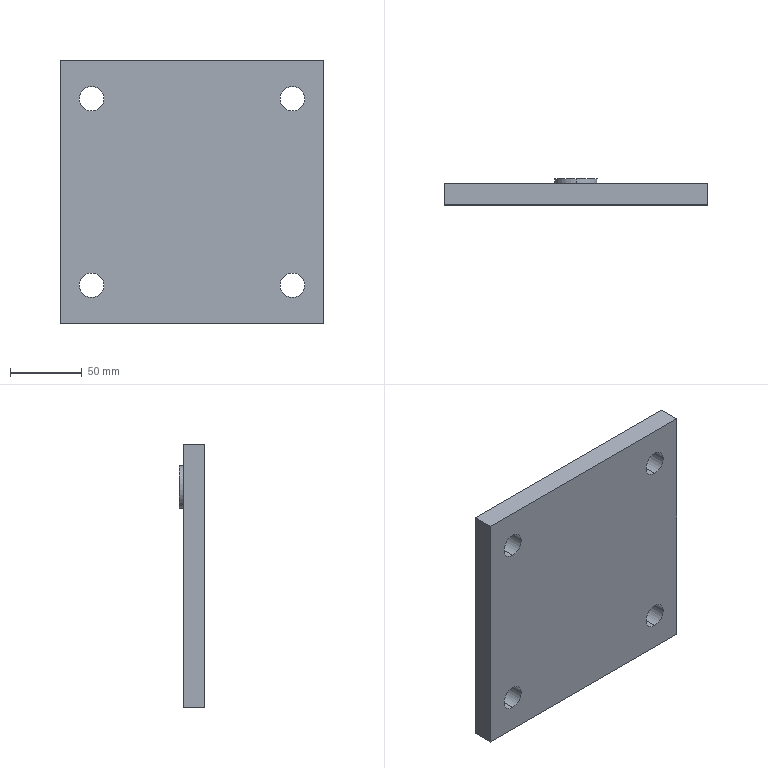Part | SolidWorks | features BaseBody 1 | 1 solid | 17 faces | box 184 x 18 x 184 mm | volume 496342 mm3 | cylinder 10 | plane 7 | commonest cylinder face diameters 17 x8 30 x2
STEP:
#1=CARTESIAN_POINT('',(70.,79.2,-206.379));
#2=VERTEX_POINT('',#1);
#3=CARTESIAN_POINT('',(70.,79.2,-223.379));
#4=VERTEX_POINT('',#3);
#5=CARTESIAN_POINT('',(70.,79.2,-214.879));
#6=DIRECTION('',(0.,-1.,0.));
#7=DIRECTION('',(0.,0.,-1.));
#8=AXIS2_PLACEMENT_3D('',#5,#6,#7);
#9=CIRCLE('',#8,8.5);
#10=EDGE_CURVE('',#2,#4,#9,.T.);
#11=ORIENTED_EDGE('',*,*,#10,.F.);
#12=CARTESIAN_POINT('',(70.,64.2,-206.379));
#13=VERTEX_POINT('',#12);
#14=CARTESIAN_POINT('',(70.,82.2,-206.379));
#15=DIRECTION('',(0.,-1.,0.));
#16=VECTOR('',#15,1000.);
#17=LINE('',#14,#16);
#18=EDGE_CURVE('',#2,#13,#17,.T.);
#19=ORIENTED_EDGE('',*,*,#18,.T.);
#20=CARTESIAN_POINT('',(70.,64.2,-223.379));
#21=VERTEX_POINT('',#20);
#22=CARTESIAN_POINT('',(70.,64.2,-214.879));
#23=DIRECTION('',(0.,-1.,0.));
#24=DIRECTION('',(0.,0.,-1.));
#25=AXIS2_PLACEMENT_3D('',#22,#23,#24);
#26=CIRCLE('',#25,8.5);
#27=EDGE_CURVE('',#13,#21,#26,.T.);
#28=ORIENTED_EDGE('',*,*,#27,.T.);
#29=CARTESIAN_POINT('',(70.,82.2,-223.379));
#30=DIRECTION('',(0.,-1.,0.));
#31=VECTOR('',#30,1000.);
#32=LINE('',#29,#31);
#33=EDGE_CURVE('',#4,#21,#32,.T.);
#34=ORIENTED_EDGE('',*,*,#33,.F.);
#35=EDGE_LOOP('',(#11,#19,#28,#34));
#36=FACE_OUTER_BOUND('',#35,.T.);
#37=CARTESIAN_POINT('',(70.,82.2,-214.879));
#38=DIRECTION('',(0.,-1.,0.));
#39=DIRECTION('',(0.,0.,-1.));
#40=AXIS2_PLACEMENT_3D('',#37,#38,#39);
#41=CYLINDRICAL_SURFACE('',#40,8.5);
#42=ADVANCED_FACE('',(#36),#41,.F.);
#43=CARTESIAN_POINT('',(70.,79.2,-76.379));
#44=VERTEX_POINT('',#43);
#45=CARTESIAN_POINT('',(70.,79.2,-93.379));
#46=VERTEX_POINT('',#45);
#47=CARTESIAN_POINT('',(70.,79.2,-84.879));
#48=DIRECTION('',(0.,-1.,0.));
#49=DIRECTION('',(0.,0.,-1.));
#50=AXIS2_PLACEMENT_3D('',#47,#48,#49);
#51=CIRCLE('',#50,8.5);
#52=EDGE_CURVE('',#44,#46,#51,.T.);
#53=ORIENTED_EDGE('',*,*,#52,.F.);
#54=CARTESIAN_POINT('',(70.,64.2,-76.379));
#55=VERTEX_POINT('',#54);
#56=CARTESIAN_POINT('',(70.,82.2,-76.379));
#57=DIRECTION('',(0.,-1.,0.));
#58=VECTOR('',#57,1000.);
#59=LINE('',#56,#58);
#60=EDGE_CURVE('',#44,#55,#59,.T.);
#61=ORIENTED_EDGE('',*,*,#60,.T.);
#62=CARTESIAN_POINT('',(70.,64.2,-93.379));
#63=VERTEX_POINT('',#62);
#64=CARTESIAN_POINT('',(70.,64.2,-84.879));
#65=DIRECTION('',(0.,-1.,0.));
#66=DIRECTION('',(0.,0.,-1.));
#67=AXIS2_PLACEMENT_3D('',#64,#65,#66);
#68=CIRCLE('',#67,8.5);
#69=EDGE_CURVE('',#55,#63,#68,.T.);
#70=ORIENTED_EDGE('',*,*,#69,.T.);
#71=CARTESIAN_POINT('',(70.,82.2,-93.379));
#72=DIRECTION('',(0.,-1.,0.));
#73=VECTOR('',#72,1000.);
#74=LINE('',#71,#73);
#75=EDGE_CURVE('',#46,#63,#74,.T.);
#76=ORIENTED_EDGE('',*,*,#75,.F.);
#77=EDGE_LOOP('',(#53,#61,#70,#76));
#78=FACE_OUTER_BOUND('',#77,.T.);
#79=CARTESIAN_POINT('',(70.,82.2,-84.879));
#80=DIRECTION('',(0.,-1.,0.));
#81=DIRECTION('',(0.,0.,-1.));
#82=AXIS2_PLACEMENT_3D('',#79,#80,#81);
#83=CYLINDRICAL_SURFACE('',#82,8.5);
#84=ADVANCED_FACE('',(#78),#83,.F.);
#85=CARTESIAN_POINT('',(-70.,79.2,-206.379));
#86=VERTEX_POINT('',#85);
#87=CARTESIAN_POINT('',(-70.,79.2,-223.379));
#88=VERTEX_POINT('',#87);
#89=CARTESIAN_POINT('',(-70.,79.2,-214.879));
#90=DIRECTION('',(0.,-1.,0.));
#91=DIRECTION('',(0.,0.,-1.));
#92=AXIS2_PLACEMENT_3D('',#89,#90,#91);
#93=CIRCLE('',#92,8.5);
#94=EDGE_CURVE('',#86,#88,#93,.T.);
#95=ORIENTED_EDGE('',*,*,#94,.F.);
#96=CARTESIAN_POINT('',(-70.,64.2,-206.379));
#97=VERTEX_POINT('',#96);
#98=CARTESIAN_POINT('',(-70.,82.2,-206.379));
#99=DIRECTION('',(0.,-1.,0.));
#100=VECTOR('',#99,1000.);
#101=LINE('',#98,#100);
#102=EDGE_CURVE('',#86,#97,#101,.T.);
#103=ORIENTED_EDGE('',*,*,#102,.T.);
#104=CARTESIAN_POINT('',(-70.,64.2,-223.379));
#105=VERTEX_POINT('',#104);
#106=CARTESIAN_POINT('',(-70.,64.2,-214.879));
#107=DIRECTION('',(0.,-1.,0.));
#108=DIRECTION('',(0.,0.,-1.));
#109=AXIS2_PLACEMENT_3D('',#106,#107,#108);
#110=CIRCLE('',#109,8.5);
#111=EDGE_CURVE('',#97,#105,#110,.T.);
#112=ORIENTED_EDGE('',*,*,#111,.T.);
#113=CARTESIAN_POINT('',(-70.,82.2,-223.379));
#114=DIRECTION('',(0.,-1.,0.));
#115=VECTOR('',#114,1000.);
#116=LINE('',#113,#115);
#117=EDGE_CURVE('',#88,#105,#116,.T.);
#118=ORIENTED_EDGE('',*,*,#117,.F.);
#119=EDGE_LOOP('',(#95,#103,#112,#118));
#120=FACE_OUTER_BOUND('',#119,.T.);
#121=CARTESIAN_POINT('',(-70.,82.2,-214.879));
#122=DIRECTION('',(0.,-1.,0.));
#123=DIRECTION('',(0.,0.,-1.));
#124=AXIS2_PLACEMENT_3D('',#121,#122,#123);
#125=CYLINDRICAL_SURFACE('',#124,8.5);
#126=ADVANCED_FACE('',(#120),#125,.F.);
#127=CARTESIAN_POINT('',(-70.,79.2,-76.379));
#128=VERTEX_POINT('',#127);
#129=CARTESIAN_POINT('',(-70.,79.2,-93.379));
#130=VERTEX_POINT('',#129);
#131=CARTESIAN_POINT('',(-70.,79.2,-84.879));
#132=DIRECTION('',(0.,-1.,0.));
#133=DIRECTION('',(0.,0.,-1.));
#134=AXIS2_PLACEMENT_3D('',#131,#132,#133);
#135=CIRCLE('',#134,8.5);
#136=EDGE_CURVE('',#128,#130,#135,.T.);
#137=ORIENTED_EDGE('',*,*,#136,.F.);
#138=CARTESIAN_POINT('',(-70.,64.2,-76.379));
#139=VERTEX_POINT('',#138);
#140=CARTESIAN_POINT('',(-70.,82.2,-76.379));
#141=DIRECTION('',(0.,-1.,0.));
#142=VECTOR('',#141,1000.);
#143=LINE('',#140,#142);
#144=EDGE_CURVE('',#128,#139,#143,.T.);
#145=ORIENTED_EDGE('',*,*,#144,.T.);
#146=CARTESIAN_POINT('',(-70.,64.2,-93.379));
#147=VERTEX_POINT('',#146);
#148=CARTESIAN_POINT('',(-70.,64.2,-84.879));
#149=DIRECTION('',(0.,-1.,0.));
#150=DIRECTION('',(0.,0.,-1.));
#151=AXIS2_PLACEMENT_3D('',#148,#149,#150);
#152=CIRCLE('',#151,8.5);
#153=EDGE_CURVE('',#139,#147,#152,.T.);
#154=ORIENTED_EDGE('',*,*,#153,.T.);
#155=CARTESIAN_POINT('',(-70.,82.2,-93.379));
#156=DIRECTION('',(0.,-1.,0.));
#157=VECTOR('',#156,1000.);
#158=LINE('',#155,#157);
#159=EDGE_CURVE('',#130,#147,#158,.T.);
#160=ORIENTED_EDGE('',*,*,#159,.F.);
#161=EDGE_LOOP('',(#137,#145,#154,#160));
#162=FACE_OUTER_BOUND('',#161,.T.);
#163=CARTESIAN_POINT('',(-70.,82.2,-84.879));
#164=DIRECTION('',(0.,-1.,0.));
#165=DIRECTION('',(0.,0.,-1.));
#166=AXIS2_PLACEMENT_3D('',#163,#164,#165);
#167=CYLINDRICAL_SURFACE('',#166,8.5);
#168=ADVANCED_FACE('',(#162),#167,.F.);
#169=CARTESIAN_POINT('',(0.,82.2,-102.879));
#170=VERTEX_POINT('',#169);
#171=CARTESIAN_POINT('',(0.,82.2,-72.879));
#172=VERTEX_POINT('',#171);
#173=CARTESIAN_POINT('',(0.,82.2,-87.879));
#174=DIRECTION('',(0.,-1.,0.));
#175=DIRECTION('',(0.,0.,-1.));
#176=AXIS2_PLACEMENT_3D('',#173,#174,#175);
#177=CIRCLE('',#176,15.);
#178=EDGE_CURVE('',#170,#172,#177,.T.);
#179=ORIENTED_EDGE('',*,*,#178,.T.);
#180=CARTESIAN_POINT('',(0.,79.2,-72.879));
#181=VERTEX_POINT('',#180);
#182=CARTESIAN_POINT('',(0.,82.2,-72.879));
#183=DIRECTION('',(0.,-1.,0.));
#184=VECTOR('',#183,1000.);
#185=LINE('',#182,#184);
#186=EDGE_CURVE('',#172,#181,#185,.T.);
#187=ORIENTED_EDGE('',*,*,#186,.T.);
#188=CARTESIAN_POINT('',(0.,79.2,-102.879));
#189=VERTEX_POINT('',#188);
#190=CARTESIAN_POINT('',(0.,79.2,-87.879));
#191=DIRECTION('',(0.,-1.,0.));
#192=DIRECTION('',(0.,0.,-1.));
#193=AXIS2_PLACEMENT_3D('',#190,#191,#192);
#194=CIRCLE('',#193,15.);
#195=EDGE_CURVE('',#189,#181,#194,.T.);
#196=ORIENTED_EDGE('',*,*,#195,.F.);
#197=CARTESIAN_POINT('',(0.,82.2,-102.879));
#198=DIRECTION('',(0.,-1.,0.));
#199=VECTOR('',#198,1000.);
#200=LINE('',#197,#199);
#201=EDGE_CURVE('',#170,#189,#200,.T.);
#202=ORIENTED_EDGE('',*,*,#201,.F.);
#203=EDGE_LOOP('',(#179,#187,#196,#202));
#204=FACE_OUTER_BOUND('',#203,.T.);
#205=CARTESIAN_POINT('',(0.,82.2,-87.879));
#206=DIRECTION('',(0.,-1.,0.));
#207=DIRECTION('',(0.,0.,-1.));
#208=AXIS2_PLACEMENT_3D('',#205,#206,#207);
#209=CYLINDRICAL_SURFACE('',#208,15.);
#210=ADVANCED_FACE('',(#204),#209,.T.);
#211=CARTESIAN_POINT('',(92.,64.2,-241.879));
#212=VERTEX_POINT('',#211);
#213=CARTESIAN_POINT('',(-92.,64.2,-241.879));
#214=VERTEX_POINT('',#213);
#215=CARTESIAN_POINT('',(0.,64.2,-241.879));
#216=DIRECTION('',(-1.,0.,0.));
#217=VECTOR('',#216,1000.);
#218=LINE('',#215,#217);
#219=EDGE_CURVE('',#212,#214,#218,.T.);
#220=ORIENTED_EDGE('',*,*,#219,.F.);
#221=CARTESIAN_POINT('',(92.,64.2,-57.879));
#222=VERTEX_POINT('',#221);
#223=CARTESIAN_POINT('',(92.,64.2,-149.879));
#224=DIRECTION('',(0.,0.,-1.));
#225=VECTOR('',#224,1000.);
#226=LINE('',#223,#225);
#227=EDGE_CURVE('',#222,#212,#226,.T.);
#228=ORIENTED_EDGE('',*,*,#227,.F.);
#229=CARTESIAN_POINT('',(-92.,64.2,-57.879));
#230=VERTEX_POINT('',#229);
#231=CARTESIAN_POINT('',(0.,64.2,-57.879));
#232=DIRECTION('',(1.,0.,0.));
#233=VECTOR('',#232,1000.);
#234=LINE('',#231,#233);
#235=EDGE_CURVE('',#230,#222,#234,.T.);
#236=ORIENTED_EDGE('',*,*,#235,.F.);
#237=CARTESIAN_POINT('',(-92.,64.2,-149.879));
#238=DIRECTION('',(0.,0.,1.));
#239=VECTOR('',#238,1000.);
#240=LINE('',#237,#239);
#241=EDGE_CURVE('',#214,#230,#240,.T.);
#242=ORIENTED_EDGE('',*,*,#241,.F.);
#243=EDGE_LOOP('',(#220,#228,#236,#242));
#244=FACE_OUTER_BOUND('',#243,.T.);
#245=CARTESIAN_POINT('',(70.,64.2,-214.879));
#246=DIRECTION('',(0.,-1.,0.));
#247=DIRECTION('',(0.,0.,-1.));
#248=AXIS2_PLACEMENT_3D('',#245,#246,#247);
#249=CIRCLE('',#248,8.5);
#250=EDGE_CURVE('',#21,#13,#249,.T.);
#251=ORIENTED_EDGE('',*,*,#250,.F.);
#252=ORIENTED_EDGE('',*,*,#27,.F.);
#253=EDGE_LOOP('',(#251,#252));
#254=FACE_BOUND('',#253,.T.);
#255=CARTESIAN_POINT('',(70.,64.2,-84.879));
#256=DIRECTION('',(0.,-1.,0.));
#257=DIRECTION('',(0.,0.,-1.));
#258=AXIS2_PLACEMENT_3D('',#255,#256,#257);
#259=CIRCLE('',#258,8.5);
#260=EDGE_CURVE('',#63,#55,#259,.T.);
#261=ORIENTED_EDGE('',*,*,#260,.F.);
#262=ORIENTED_EDGE('',*,*,#69,.F.);
#263=EDGE_LOOP('',(#261,#262));
#264=FACE_BOUND('',#263,.T.);
#265=CARTESIAN_POINT('',(-70.,64.2,-214.879));
#266=DIRECTION('',(0.,-1.,0.));
#267=DIRECTION('',(0.,0.,-1.));
#268=AXIS2_PLACEMENT_3D('',#265,#266,#267);
#269=CIRCLE('',#268,8.5);
#270=EDGE_CURVE('',#105,#97,#269,.T.);
#271=ORIENTED_EDGE('',*,*,#270,.F.);
#272=ORIENTED_EDGE('',*,*,#111,.F.);
#273=EDGE_LOOP('',(#271,#272));
#274=FACE_BOUND('',#273,.T.);
#275=CARTESIAN_POINT('',(-70.,64.2,-84.879));
#276=DIRECTION('',(0.,-1.,0.));
#277=DIRECTION('',(0.,0.,-1.));
#278=AXIS2_PLACEMENT_3D('',#275,#276,#277);
#279=CIRCLE('',#278,8.5);
#280=EDGE_CURVE('',#147,#139,#279,.T.);
#281=ORIENTED_EDGE('',*,*,#280,.F.);
#282=ORIENTED_EDGE('',*,*,#153,.F.);
#283=EDGE_LOOP('',(#281,#282));
#284=FACE_BOUND('',#283,.T.);
#285=CARTESIAN_POINT('',(0.,64.2,-149.879));
#286=DIRECTION('',(0.,1.,0.));
#287=DIRECTION('',(0.,0.,1.));
#288=AXIS2_PLACEMENT_3D('',#285,#286,#287);
#289=PLANE('',#288);
#290=ADVANCED_FACE('',(#244,#254,#264,#274,#284),#289,.F.);
#291=CARTESIAN_POINT('',(-92.,79.2,-57.879));
#292=VERTEX_POINT('',#291);
#293=CARTESIAN_POINT('',(-92.,79.2,-57.879));
#294=DIRECTION('',(0.,-1.,0.));
#295=VECTOR('',#294,1000.);
#296=LINE('',#293,#295);
#297=EDGE_CURVE('',#292,#230,#296,.T.);
#298=ORIENTED_EDGE('',*,*,#297,.F.);
#299=CARTESIAN_POINT('',(-92.,79.2,-241.879));
#300=VERTEX_POINT('',#299);
#301=CARTESIAN_POINT('',(-92.,79.2,-57.879));
#302=DIRECTION('',(0.,0.,1.));
#303=VECTOR('',#302,1000.);
#304=LINE('',#301,#303);
#305=EDGE_CURVE('',#300,#292,#304,.T.);
#306=ORIENTED_EDGE('',*,*,#305,.F.);
#307=CARTESIAN_POINT('',(-92.,79.2,-241.879));
#308=DIRECTION('',(0.,1.,0.));
#309=VECTOR('',#308,1000.);
#310=LINE('',#307,#309);
#311=EDGE_CURVE('',#214,#300,#310,.T.);
#312=ORIENTED_EDGE('',*,*,#311,.F.);
#313=ORIENTED_EDGE('',*,*,#241,.T.);
#314=EDGE_LOOP('',(#298,#306,#312,#313));
#315=FACE_OUTER_BOUND('',#314,.T.);
#316=CARTESIAN_POINT('',(-92.,79.2,-57.879));
#317=DIRECTION('',(1.,0.,0.));
#318=DIRECTION('',(0.,0.,-1.));
#319=AXIS2_PLACEMENT_3D('',#316,#317,#318);
#320=PLANE('',#319);
#321=ADVANCED_FACE('',(#315),#320,.F.);
#322=ORIENTED_EDGE('',*,*,#311,.T.);
#323=CARTESIAN_POINT('',(92.,79.2,-241.879));
#324=VERTEX_POINT('',#323);
#325=CARTESIAN_POINT('',(92.,79.2,-241.879));
#326=DIRECTION('',(-1.,0.,0.));
#327=VECTOR('',#326,1000.);
#328=LINE('',#325,#327);
#329=EDGE_CURVE('',#324,#300,#328,.T.);
#330=ORIENTED_EDGE('',*,*,#329,.F.);
#331=CARTESIAN_POINT('',(92.,79.2,-241.879));
#332=DIRECTION('',(0.,1.,0.));
#333=VECTOR('',#332,1000.);
#334=LINE('',#331,#333);
#335=EDGE_CURVE('',#212,#324,#334,.T.);
#336=ORIENTED_EDGE('',*,*,#335,.F.);
#337=ORIENTED_EDGE('',*,*,#219,.T.);
#338=EDGE_LOOP('',(#322,#330,#336,#337));
#339=FACE_OUTER_BOUND('',#338,.T.);
#340=CARTESIAN_POINT('',(92.,79.2,-241.879));
#341=DIRECTION('',(0.,0.,1.));
#342=DIRECTION('',(1.,0.,0.));
#343=AXIS2_PLACEMENT_3D('',#340,#341,#342);
#344=PLANE('',#343);
#345=ADVANCED_FACE('',(#339),#344,.F.);
#346=ORIENTED_EDGE('',*,*,#335,.T.);
#347=CARTESIAN_POINT('',(92.,79.2,-57.879));
#348=VERTEX_POINT('',#347);
#349=CARTESIAN_POINT('',(92.,79.2,-57.879));
#350=DIRECTION('',(0.,0.,-1.));
#351=VECTOR('',#350,1000.);
#352=LINE('',#349,#351);
#353=EDGE_CURVE('',#348,#324,#352,.T.);
#354=ORIENTED_EDGE('',*,*,#353,.F.);
#355=CARTESIAN_POINT('',(92.,79.2,-57.879));
#356=DIRECTION('',(0.,1.,0.));
#357=VECTOR('',#356,1000.);
#358=LINE('',#355,#357);
#359=EDGE_CURVE('',#222,#348,#358,.T.);
#360=ORIENTED_EDGE('',*,*,#359,.F.);
#361=ORIENTED_EDGE('',*,*,#227,.T.);
#362=EDGE_LOOP('',(#346,#354,#360,#361));
#363=FACE_OUTER_BOUND('',#362,.T.);
#364=CARTESIAN_POINT('',(92.,79.2,-57.879));
#365=DIRECTION('',(-1.,0.,0.));
#366=DIRECTION('',(0.,0.,1.));
#367=AXIS2_PLACEMENT_3D('',#364,#365,#366);
#368=PLANE('',#367);
#369=ADVANCED_FACE('',(#363),#368,.F.);
#370=ORIENTED_EDGE('',*,*,#359,.T.);
#371=CARTESIAN_POINT('',(92.,79.2,-57.879));
#372=DIRECTION('',(1.,0.,0.));
#373=VECTOR('',#372,1000.);
#374=LINE('',#371,#373);
#375=EDGE_CURVE('',#292,#348,#374,.T.);
#376=ORIENTED_EDGE('',*,*,#375,.F.);
#377=ORIENTED_EDGE('',*,*,#297,.T.);
#378=ORIENTED_EDGE('',*,*,#235,.T.);
#379=EDGE_LOOP('',(#370,#376,#377,#378));
#380=FACE_OUTER_BOUND('',#379,.T.);
#381=CARTESIAN_POINT('',(92.,79.2,-57.879));
#382=DIRECTION('',(0.,0.,-1.));
#383=DIRECTION('',(-1.,0.,0.));
#384=AXIS2_PLACEMENT_3D('',#381,#382,#383);
#385=PLANE('',#384);
#386=ADVANCED_FACE('',(#380),#385,.F.);
#387=ORIENTED_EDGE('',*,*,#18,.F.);
#388=CARTESIAN_POINT('',(70.,79.2,-214.879));
#389=DIRECTION('',(0.,-1.,0.));
#390=DIRECTION('',(0.,0.,-1.));
#391=AXIS2_PLACEMENT_3D('',#388,#389,#390);
#392=CIRCLE('',#391,8.5);
#393=EDGE_CURVE('',#4,#2,#392,.T.);
#394=ORIENTED_EDGE('',*,*,#393,.F.);
#395=ORIENTED_EDGE('',*,*,#33,.T.);
#396=ORIENTED_EDGE('',*,*,#250,.T.);
#397=EDGE_LOOP('',(#387,#394,#395,#396));
#398=FACE_OUTER_BOUND('',#397,.T.);
#399=CARTESIAN_POINT('',(70.,82.2,-214.879));
#400=DIRECTION('',(0.,-1.,0.));
#401=DIRECTION('',(0.,0.,-1.));
#402=AXIS2_PLACEMENT_3D('',#399,#400,#401);
#403=CYLINDRICAL_SURFACE('',#402,8.5);
#404=ADVANCED_FACE('',(#398),#403,.F.);
#405=ORIENTED_EDGE('',*,*,#60,.F.);
#406=CARTESIAN_POINT('',(70.,79.2,-84.879));
#407=DIRECTION('',(0.,-1.,0.));
#408=DIRECTION('',(0.,0.,-1.));
#409=AXIS2_PLACEMENT_3D('',#406,#407,#408);
#410=CIRCLE('',#409,8.5);
#411=EDGE_CURVE('',#46,#44,#410,.T.);
#412=ORIENTED_EDGE('',*,*,#411,.F.);
#413=ORIENTED_EDGE('',*,*,#75,.T.);
#414=ORIENTED_EDGE('',*,*,#260,.T.);
#415=EDGE_LOOP('',(#405,#412,#413,#414));
#416=FACE_OUTER_BOUND('',#415,.T.);
#417=CARTESIAN_POINT('',(70.,82.2,-84.879));
#418=DIRECTION('',(0.,-1.,0.));
#419=DIRECTION('',(0.,0.,-1.));
#420=AXIS2_PLACEMENT_3D('',#417,#418,#419);
#421=CYLINDRICAL_SURFACE('',#420,8.5);
#422=ADVANCED_FACE('',(#416),#421,.F.);
#423=ORIENTED_EDGE('',*,*,#102,.F.);
#424=CARTESIAN_POINT('',(-70.,79.2,-214.879));
#425=DIRECTION('',(0.,-1.,0.));
#426=DIRECTION('',(0.,0.,-1.));
#427=AXIS2_PLACEMENT_3D('',#424,#425,#426);
#428=CIRCLE('',#427,8.5);
#429=EDGE_CURVE('',#88,#86,#428,.T.);
#430=ORIENTED_EDGE('',*,*,#429,.F.);
#431=ORIENTED_EDGE('',*,*,#117,.T.);
#432=ORIENTED_EDGE('',*,*,#270,.T.);
#433=EDGE_LOOP('',(#423,#430,#431,#432));
#434=FACE_OUTER_BOUND('',#433,.T.);
#435=CARTESIAN_POINT('',(-70.,82.2,-214.879));
#436=DIRECTION('',(0.,-1.,0.));
#437=DIRECTION('',(0.,0.,-1.));
#438=AXIS2_PLACEMENT_3D('',#435,#436,#437);
#439=CYLINDRICAL_SURFACE('',#438,8.5);
#440=ADVANCED_FACE('',(#434),#439,.F.);
#441=ORIENTED_EDGE('',*,*,#144,.F.);
#442=CARTESIAN_POINT('',(-70.,79.2,-84.879));
#443=DIRECTION('',(0.,-1.,0.));
#444=DIRECTION('',(0.,0.,-1.));
#445=AXIS2_PLACEMENT_3D('',#442,#443,#444);
#446=CIRCLE('',#445,8.5);
#447=EDGE_CURVE('',#130,#128,#446,.T.);
#448=ORIENTED_EDGE('',*,*,#447,.F.);
#449=ORIENTED_EDGE('',*,*,#159,.T.);
#450=ORIENTED_EDGE('',*,*,#280,.T.);
#451=EDGE_LOOP('',(#441,#448,#449,#450));
#452=FACE_OUTER_BOUND('',#451,.T.);
#453=CARTESIAN_POINT('',(-70.,82.2,-84.879));
#454=DIRECTION('',(0.,-1.,0.));
#455=DIRECTION('',(0.,0.,-1.));
#456=AXIS2_PLACEMENT_3D('',#453,#454,#455);
#457=CYLINDRICAL_SURFACE('',#456,8.5);
#458=ADVANCED_FACE('',(#452),#457,.F.);
#459=ORIENTED_EDGE('',*,*,#195,.T.);
#460=CARTESIAN_POINT('',(0.,79.2,-87.879));
#461=DIRECTION('',(0.,-1.,0.));
#462=DIRECTION('',(0.,0.,-1.));
#463=AXIS2_PLACEMENT_3D('',#460,#461,#462);
#464=CIRCLE('',#463,15.);
#465=EDGE_CURVE('',#181,#189,#464,.T.);
#466=ORIENTED_EDGE('',*,*,#465,.T.);
#467=EDGE_LOOP('',(#459,#466));
#468=FACE_BOUND('',#467,.T.);
#469=ORIENTED_EDGE('',*,*,#353,.T.);
#470=ORIENTED_EDGE('',*,*,#329,.T.);
#471=ORIENTED_EDGE('',*,*,#305,.T.);
#472=ORIENTED_EDGE('',*,*,#375,.T.);
#473=EDGE_LOOP('',(#469,#470,#471,#472));
#474=FACE_OUTER_BOUND('',#473,.T.);
#475=ORIENTED_EDGE('',*,*,#393,.T.);
#476=ORIENTED_EDGE('',*,*,#10,.T.);
#477=EDGE_LOOP('',(#475,#476));
#478=FACE_BOUND('',#477,.T.);
#479=ORIENTED_EDGE('',*,*,#411,.T.);
#480=ORIENTED_EDGE('',*,*,#52,.T.);
#481=EDGE_LOOP('',(#479,#480));
#482=FACE_BOUND('',#481,.T.);
#483=ORIENTED_EDGE('',*,*,#429,.T.);
#484=ORIENTED_EDGE('',*,*,#94,.T.);
#485=EDGE_LOOP('',(#483,#484));
#486=FACE_BOUND('',#485,.T.);
#487=ORIENTED_EDGE('',*,*,#447,.T.);
#488=ORIENTED_EDGE('',*,*,#136,.T.);
#489=EDGE_LOOP('',(#487,#488));
#490=FACE_BOUND('',#489,.T.);
#491=CARTESIAN_POINT('',(0.,79.2,-149.879));
#492=DIRECTION('',(0.,1.,0.));
#493=DIRECTION('',(0.,0.,1.));
#494=AXIS2_PLACEMENT_3D('',#491,#492,#493);
#495=PLANE('',#494);
#496=ADVANCED_FACE('',(#468,#474,#478,#482,#486,#490),#495,.T.);
#497=ORIENTED_EDGE('',*,*,#186,.F.);
#498=CARTESIAN_POINT('',(0.,82.2,-87.879));
#499=DIRECTION('',(0.,-1.,0.));
#500=DIRECTION('',(0.,0.,-1.));
#501=AXIS2_PLACEMENT_3D('',#498,#499,#500);
#502=CIRCLE('',#501,15.);
#503=EDGE_CURVE('',#172,#170,#502,.T.);
#504=ORIENTED_EDGE('',*,*,#503,.T.);
#505=ORIENTED_EDGE('',*,*,#201,.T.);
#506=ORIENTED_EDGE('',*,*,#465,.F.);
#507=EDGE_LOOP('',(#497,#504,#505,#506));
#508=FACE_OUTER_BOUND('',#507,.T.);
#509=CARTESIAN_POINT('',(0.,82.2,-87.879));
#510=DIRECTION('',(0.,-1.,0.));
#511=DIRECTION('',(0.,0.,-1.));
#512=AXIS2_PLACEMENT_3D('',#509,#510,#511);
#513=CYLINDRICAL_SURFACE('',#512,15.);
#514=ADVANCED_FACE('',(#508),#513,.T.);
#515=ORIENTED_EDGE('',*,*,#178,.F.);
#516=ORIENTED_EDGE('',*,*,#503,.F.);
#517=EDGE_LOOP('',(#515,#516));
#518=FACE_OUTER_BOUND('',#517,.T.);
#519=CARTESIAN_POINT('',(0.,82.2,-87.879));
#520=DIRECTION('',(0.,1.,0.));
#521=DIRECTION('',(0.,0.,1.));
#522=AXIS2_PLACEMENT_3D('',#519,#520,#521);
#523=PLANE('',#522);
#524=ADVANCED_FACE('',(#518),#523,.T.);
#525=CLOSED_SHELL('',(#42,#84,#126,#168,#210,#290,#321,#345,#369,#386,#404,#422,#440,#458,#496,#514,#524));
#526=MANIFOLD_SOLID_BREP('',#525);
#527=CARTESIAN_POINT('',(0.,0.,0.));
#528=DIRECTION('',(0.,0.,1.));
#529=DIRECTION('',(1.,0.,0.));
#530=AXIS2_PLACEMENT_3D('',#527,#528,#529);
#531=(LENGTH_UNIT()NAMED_UNIT(*)SI_UNIT(.MILLI.,.METRE.));
#532=UNCERTAINTY_MEASURE_WITH_UNIT(LENGTH_MEASURE(0.00001),#531,'','');
#533=(NAMED_UNIT(*)PLANE_ANGLE_UNIT()SI_UNIT($,.RADIAN.));
#534=(NAMED_UNIT(*)SI_UNIT($,.STERADIAN.)SOLID_ANGLE_UNIT());
#535=(GEOMETRIC_REPRESENTATION_CONTEXT(3)GLOBAL_UNCERTAINTY_ASSIGNED_CONTEXT((#532))GLOBAL_UNIT_ASSIGNED_CONTEXT((#531,#533,#534))REPRESENTATION_CONTEXT('',''));
#536=ADVANCED_BREP_SHAPE_REPRESENTATION('',(#526,#530),#535);